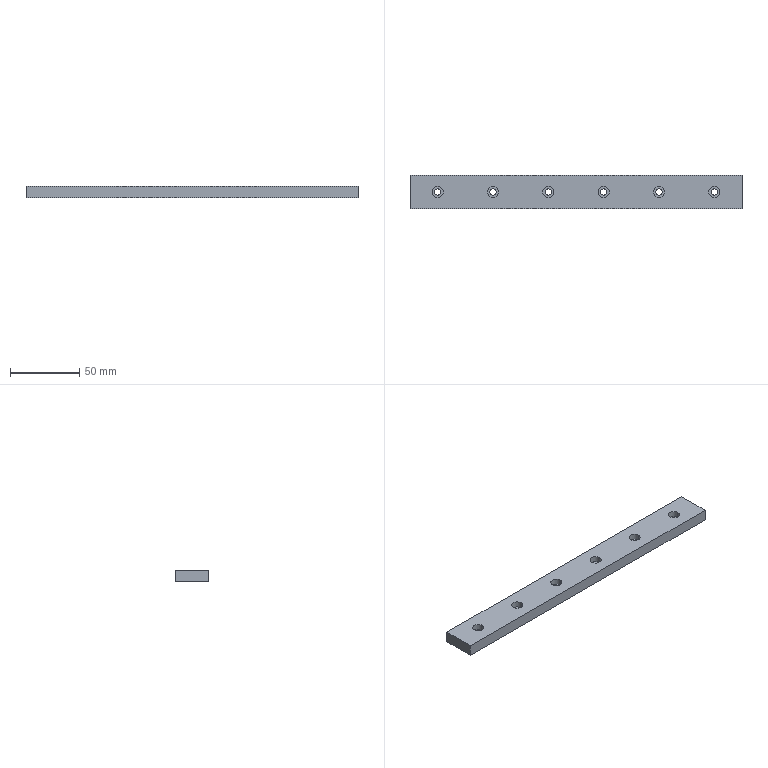Part | SolidWorks | features Extrusion 1, HoleWzd 1, LPattern 1 | 1 solid | 36 faces | box 240 x 24 x 8.5 mm | volume 47242 mm3 | cylinder 24 | plane 12 | commonest cylinder face diameters 4.5 x12 8 x12
STEP:
#1=CARTESIAN_POINT('',(96.,0.,4.1));
#2=VERTEX_POINT('',#1);
#3=CARTESIAN_POINT('',(104.,0.,4.1));
#4=VERTEX_POINT('',#3);
#5=CARTESIAN_POINT('',(100.,0.,4.1));
#6=DIRECTION('',(0.,0.,1.));
#7=DIRECTION('',(1.,0.,0.));
#8=AXIS2_PLACEMENT_3D('',#5,#6,#7);
#9=CIRCLE('',#8,4.);
#10=EDGE_CURVE('',#2,#4,#9,.T.);
#11=ORIENTED_EDGE('',*,*,#10,.F.);
#12=CARTESIAN_POINT('',(96.,0.,8.5));
#13=VERTEX_POINT('',#12);
#14=CARTESIAN_POINT('',(96.,0.,8.5));
#15=DIRECTION('',(0.,0.,1.));
#16=VECTOR('',#15,1000.);
#17=LINE('',#14,#16);
#18=EDGE_CURVE('',#2,#13,#17,.T.);
#19=ORIENTED_EDGE('',*,*,#18,.T.);
#20=CARTESIAN_POINT('',(104.,0.,8.5));
#21=VERTEX_POINT('',#20);
#22=CARTESIAN_POINT('',(100.,0.,8.5));
#23=DIRECTION('',(0.,0.,1.));
#24=DIRECTION('',(1.,0.,0.));
#25=AXIS2_PLACEMENT_3D('',#22,#23,#24);
#26=CIRCLE('',#25,4.);
#27=EDGE_CURVE('',#13,#21,#26,.T.);
#28=ORIENTED_EDGE('',*,*,#27,.T.);
#29=CARTESIAN_POINT('',(104.,0.,8.5));
#30=DIRECTION('',(0.,0.,1.));
#31=VECTOR('',#30,1000.);
#32=LINE('',#29,#31);
#33=EDGE_CURVE('',#4,#21,#32,.T.);
#34=ORIENTED_EDGE('',*,*,#33,.F.);
#35=EDGE_LOOP('',(#11,#19,#28,#34));
#36=FACE_OUTER_BOUND('',#35,.T.);
#37=CARTESIAN_POINT('',(100.,0.,8.5));
#38=DIRECTION('',(0.,0.,1.));
#39=DIRECTION('',(1.,0.,0.));
#40=AXIS2_PLACEMENT_3D('',#37,#38,#39);
#41=CYLINDRICAL_SURFACE('',#40,4.);
#42=ADVANCED_FACE('',(#36),#41,.F.);
#43=CARTESIAN_POINT('',(97.75,0.,0.));
#44=VERTEX_POINT('',#43);
#45=CARTESIAN_POINT('',(102.25,0.,0.));
#46=VERTEX_POINT('',#45);
#47=CARTESIAN_POINT('',(100.,0.,0.));
#48=DIRECTION('',(0.,0.,1.));
#49=DIRECTION('',(1.,0.,0.));
#50=AXIS2_PLACEMENT_3D('',#47,#48,#49);
#51=CIRCLE('',#50,2.25);
#52=EDGE_CURVE('',#44,#46,#51,.T.);
#53=ORIENTED_EDGE('',*,*,#52,.F.);
#54=CARTESIAN_POINT('',(97.75,0.,4.1));
#55=VERTEX_POINT('',#54);
#56=CARTESIAN_POINT('',(97.75,0.,8.5));
#57=DIRECTION('',(0.,0.,1.));
#58=VECTOR('',#57,1000.);
#59=LINE('',#56,#58);
#60=EDGE_CURVE('',#44,#55,#59,.T.);
#61=ORIENTED_EDGE('',*,*,#60,.T.);
#62=CARTESIAN_POINT('',(102.25,0.,4.1));
#63=VERTEX_POINT('',#62);
#64=CARTESIAN_POINT('',(100.,0.,4.1));
#65=DIRECTION('',(0.,0.,1.));
#66=DIRECTION('',(1.,0.,0.));
#67=AXIS2_PLACEMENT_3D('',#64,#65,#66);
#68=CIRCLE('',#67,2.25);
#69=EDGE_CURVE('',#55,#63,#68,.T.);
#70=ORIENTED_EDGE('',*,*,#69,.T.);
#71=CARTESIAN_POINT('',(102.25,0.,8.5));
#72=DIRECTION('',(0.,0.,1.));
#73=VECTOR('',#72,1000.);
#74=LINE('',#71,#73);
#75=EDGE_CURVE('',#46,#63,#74,.T.);
#76=ORIENTED_EDGE('',*,*,#75,.F.);
#77=EDGE_LOOP('',(#53,#61,#70,#76));
#78=FACE_OUTER_BOUND('',#77,.T.);
#79=CARTESIAN_POINT('',(100.,0.,8.5));
#80=DIRECTION('',(0.,0.,1.));
#81=DIRECTION('',(1.,0.,0.));
#82=AXIS2_PLACEMENT_3D('',#79,#80,#81);
#83=CYLINDRICAL_SURFACE('',#82,2.25);
#84=ADVANCED_FACE('',(#78),#83,.F.);
#85=CARTESIAN_POINT('',(56.,0.,4.1));
#86=VERTEX_POINT('',#85);
#87=CARTESIAN_POINT('',(64.,0.,4.1));
#88=VERTEX_POINT('',#87);
#89=CARTESIAN_POINT('',(60.,0.,4.1));
#90=DIRECTION('',(0.,0.,1.));
#91=DIRECTION('',(1.,0.,0.));
#92=AXIS2_PLACEMENT_3D('',#89,#90,#91);
#93=CIRCLE('',#92,4.);
#94=EDGE_CURVE('',#86,#88,#93,.T.);
#95=ORIENTED_EDGE('',*,*,#94,.F.);
#96=CARTESIAN_POINT('',(56.,0.,8.5));
#97=VERTEX_POINT('',#96);
#98=CARTESIAN_POINT('',(56.,0.,8.5));
#99=DIRECTION('',(0.,0.,1.));
#100=VECTOR('',#99,1000.);
#101=LINE('',#98,#100);
#102=EDGE_CURVE('',#86,#97,#101,.T.);
#103=ORIENTED_EDGE('',*,*,#102,.T.);
#104=CARTESIAN_POINT('',(64.,0.,8.5));
#105=VERTEX_POINT('',#104);
#106=CARTESIAN_POINT('',(60.,0.,8.5));
#107=DIRECTION('',(0.,0.,1.));
#108=DIRECTION('',(1.,0.,0.));
#109=AXIS2_PLACEMENT_3D('',#106,#107,#108);
#110=CIRCLE('',#109,4.);
#111=EDGE_CURVE('',#97,#105,#110,.T.);
#112=ORIENTED_EDGE('',*,*,#111,.T.);
#113=CARTESIAN_POINT('',(64.,0.,8.5));
#114=DIRECTION('',(0.,0.,1.));
#115=VECTOR('',#114,1000.);
#116=LINE('',#113,#115);
#117=EDGE_CURVE('',#88,#105,#116,.T.);
#118=ORIENTED_EDGE('',*,*,#117,.F.);
#119=EDGE_LOOP('',(#95,#103,#112,#118));
#120=FACE_OUTER_BOUND('',#119,.T.);
#121=CARTESIAN_POINT('',(60.,0.,8.5));
#122=DIRECTION('',(0.,0.,1.));
#123=DIRECTION('',(1.,0.,0.));
#124=AXIS2_PLACEMENT_3D('',#121,#122,#123);
#125=CYLINDRICAL_SURFACE('',#124,4.);
#126=ADVANCED_FACE('',(#120),#125,.F.);
#127=CARTESIAN_POINT('',(57.75,0.,0.));
#128=VERTEX_POINT('',#127);
#129=CARTESIAN_POINT('',(62.25,0.,0.));
#130=VERTEX_POINT('',#129);
#131=CARTESIAN_POINT('',(60.,0.,0.));
#132=DIRECTION('',(0.,0.,1.));
#133=DIRECTION('',(1.,0.,0.));
#134=AXIS2_PLACEMENT_3D('',#131,#132,#133);
#135=CIRCLE('',#134,2.25);
#136=EDGE_CURVE('',#128,#130,#135,.T.);
#137=ORIENTED_EDGE('',*,*,#136,.F.);
#138=CARTESIAN_POINT('',(57.75,0.,4.1));
#139=VERTEX_POINT('',#138);
#140=CARTESIAN_POINT('',(57.75,0.,8.5));
#141=DIRECTION('',(0.,0.,1.));
#142=VECTOR('',#141,1000.);
#143=LINE('',#140,#142);
#144=EDGE_CURVE('',#128,#139,#143,.T.);
#145=ORIENTED_EDGE('',*,*,#144,.T.);
#146=CARTESIAN_POINT('',(62.25,0.,4.1));
#147=VERTEX_POINT('',#146);
#148=CARTESIAN_POINT('',(60.,0.,4.1));
#149=DIRECTION('',(0.,0.,1.));
#150=DIRECTION('',(1.,0.,0.));
#151=AXIS2_PLACEMENT_3D('',#148,#149,#150);
#152=CIRCLE('',#151,2.25);
#153=EDGE_CURVE('',#139,#147,#152,.T.);
#154=ORIENTED_EDGE('',*,*,#153,.T.);
#155=CARTESIAN_POINT('',(62.25,0.,8.5));
#156=DIRECTION('',(0.,0.,1.));
#157=VECTOR('',#156,1000.);
#158=LINE('',#155,#157);
#159=EDGE_CURVE('',#130,#147,#158,.T.);
#160=ORIENTED_EDGE('',*,*,#159,.F.);
#161=EDGE_LOOP('',(#137,#145,#154,#160));
#162=FACE_OUTER_BOUND('',#161,.T.);
#163=CARTESIAN_POINT('',(60.,0.,8.5));
#164=DIRECTION('',(0.,0.,1.));
#165=DIRECTION('',(1.,0.,0.));
#166=AXIS2_PLACEMENT_3D('',#163,#164,#165);
#167=CYLINDRICAL_SURFACE('',#166,2.25);
#168=ADVANCED_FACE('',(#162),#167,.F.);
#169=CARTESIAN_POINT('',(16.,0.,4.1));
#170=VERTEX_POINT('',#169);
#171=CARTESIAN_POINT('',(24.,0.,4.1));
#172=VERTEX_POINT('',#171);
#173=CARTESIAN_POINT('',(20.,0.,4.1));
#174=DIRECTION('',(0.,0.,1.));
#175=DIRECTION('',(1.,0.,0.));
#176=AXIS2_PLACEMENT_3D('',#173,#174,#175);
#177=CIRCLE('',#176,4.);
#178=EDGE_CURVE('',#170,#172,#177,.T.);
#179=ORIENTED_EDGE('',*,*,#178,.F.);
#180=CARTESIAN_POINT('',(16.,0.,8.5));
#181=VERTEX_POINT('',#180);
#182=CARTESIAN_POINT('',(16.,0.,8.5));
#183=DIRECTION('',(0.,0.,1.));
#184=VECTOR('',#183,1000.);
#185=LINE('',#182,#184);
#186=EDGE_CURVE('',#170,#181,#185,.T.);
#187=ORIENTED_EDGE('',*,*,#186,.T.);
#188=CARTESIAN_POINT('',(24.,0.,8.5));
#189=VERTEX_POINT('',#188);
#190=CARTESIAN_POINT('',(20.,0.,8.5));
#191=DIRECTION('',(0.,0.,1.));
#192=DIRECTION('',(1.,0.,0.));
#193=AXIS2_PLACEMENT_3D('',#190,#191,#192);
#194=CIRCLE('',#193,4.);
#195=EDGE_CURVE('',#181,#189,#194,.T.);
#196=ORIENTED_EDGE('',*,*,#195,.T.);
#197=CARTESIAN_POINT('',(24.,0.,8.5));
#198=DIRECTION('',(0.,0.,1.));
#199=VECTOR('',#198,1000.);
#200=LINE('',#197,#199);
#201=EDGE_CURVE('',#172,#189,#200,.T.);
#202=ORIENTED_EDGE('',*,*,#201,.F.);
#203=EDGE_LOOP('',(#179,#187,#196,#202));
#204=FACE_OUTER_BOUND('',#203,.T.);
#205=CARTESIAN_POINT('',(20.,0.,8.5));
#206=DIRECTION('',(0.,0.,1.));
#207=DIRECTION('',(1.,0.,0.));
#208=AXIS2_PLACEMENT_3D('',#205,#206,#207);
#209=CYLINDRICAL_SURFACE('',#208,4.);
#210=ADVANCED_FACE('',(#204),#209,.F.);
#211=CARTESIAN_POINT('',(17.75,0.,0.));
#212=VERTEX_POINT('',#211);
#213=CARTESIAN_POINT('',(22.25,0.,0.));
#214=VERTEX_POINT('',#213);
#215=CARTESIAN_POINT('',(20.,0.,0.));
#216=DIRECTION('',(0.,0.,1.));
#217=DIRECTION('',(1.,0.,0.));
#218=AXIS2_PLACEMENT_3D('',#215,#216,#217);
#219=CIRCLE('',#218,2.25);
#220=EDGE_CURVE('',#212,#214,#219,.T.);
#221=ORIENTED_EDGE('',*,*,#220,.F.);
#222=CARTESIAN_POINT('',(17.75,0.,4.1));
#223=VERTEX_POINT('',#222);
#224=CARTESIAN_POINT('',(17.75,0.,8.5));
#225=DIRECTION('',(0.,0.,1.));
#226=VECTOR('',#225,1000.);
#227=LINE('',#224,#226);
#228=EDGE_CURVE('',#212,#223,#227,.T.);
#229=ORIENTED_EDGE('',*,*,#228,.T.);
#230=CARTESIAN_POINT('',(22.25,0.,4.1));
#231=VERTEX_POINT('',#230);
#232=CARTESIAN_POINT('',(20.,0.,4.1));
#233=DIRECTION('',(0.,0.,1.));
#234=DIRECTION('',(1.,0.,0.));
#235=AXIS2_PLACEMENT_3D('',#232,#233,#234);
#236=CIRCLE('',#235,2.25);
#237=EDGE_CURVE('',#223,#231,#236,.T.);
#238=ORIENTED_EDGE('',*,*,#237,.T.);
#239=CARTESIAN_POINT('',(22.25,0.,8.5));
#240=DIRECTION('',(0.,0.,1.));
#241=VECTOR('',#240,1000.);
#242=LINE('',#239,#241);
#243=EDGE_CURVE('',#214,#231,#242,.T.);
#244=ORIENTED_EDGE('',*,*,#243,.F.);
#245=EDGE_LOOP('',(#221,#229,#238,#244));
#246=FACE_OUTER_BOUND('',#245,.T.);
#247=CARTESIAN_POINT('',(20.,0.,8.5));
#248=DIRECTION('',(0.,0.,1.));
#249=DIRECTION('',(1.,0.,0.));
#250=AXIS2_PLACEMENT_3D('',#247,#248,#249);
#251=CYLINDRICAL_SURFACE('',#250,2.25);
#252=ADVANCED_FACE('',(#246),#251,.F.);
#253=CARTESIAN_POINT('',(-24.,0.,4.1));
#254=VERTEX_POINT('',#253);
#255=CARTESIAN_POINT('',(-16.,0.,4.1));
#256=VERTEX_POINT('',#255);
#257=CARTESIAN_POINT('',(-20.,0.,4.1));
#258=DIRECTION('',(0.,0.,1.));
#259=DIRECTION('',(1.,0.,0.));
#260=AXIS2_PLACEMENT_3D('',#257,#258,#259);
#261=CIRCLE('',#260,4.);
#262=EDGE_CURVE('',#254,#256,#261,.T.);
#263=ORIENTED_EDGE('',*,*,#262,.F.);
#264=CARTESIAN_POINT('',(-24.,0.,8.5));
#265=VERTEX_POINT('',#264);
#266=CARTESIAN_POINT('',(-24.,0.,8.5));
#267=DIRECTION('',(0.,0.,1.));
#268=VECTOR('',#267,1000.);
#269=LINE('',#266,#268);
#270=EDGE_CURVE('',#254,#265,#269,.T.);
#271=ORIENTED_EDGE('',*,*,#270,.T.);
#272=CARTESIAN_POINT('',(-16.,0.,8.5));
#273=VERTEX_POINT('',#272);
#274=CARTESIAN_POINT('',(-20.,0.,8.5));
#275=DIRECTION('',(0.,0.,1.));
#276=DIRECTION('',(1.,0.,0.));
#277=AXIS2_PLACEMENT_3D('',#274,#275,#276);
#278=CIRCLE('',#277,4.);
#279=EDGE_CURVE('',#265,#273,#278,.T.);
#280=ORIENTED_EDGE('',*,*,#279,.T.);
#281=CARTESIAN_POINT('',(-16.,0.,8.5));
#282=DIRECTION('',(0.,0.,1.));
#283=VECTOR('',#282,1000.);
#284=LINE('',#281,#283);
#285=EDGE_CURVE('',#256,#273,#284,.T.);
#286=ORIENTED_EDGE('',*,*,#285,.F.);
#287=EDGE_LOOP('',(#263,#271,#280,#286));
#288=FACE_OUTER_BOUND('',#287,.T.);
#289=CARTESIAN_POINT('',(-20.,0.,8.5));
#290=DIRECTION('',(0.,0.,1.));
#291=DIRECTION('',(1.,0.,0.));
#292=AXIS2_PLACEMENT_3D('',#289,#290,#291);
#293=CYLINDRICAL_SURFACE('',#292,4.);
#294=ADVANCED_FACE('',(#288),#293,.F.);
#295=CARTESIAN_POINT('',(-22.25,0.,0.));
#296=VERTEX_POINT('',#295);
#297=CARTESIAN_POINT('',(-17.75,0.,0.));
#298=VERTEX_POINT('',#297);
#299=CARTESIAN_POINT('',(-20.,0.,0.));
#300=DIRECTION('',(0.,0.,1.));
#301=DIRECTION('',(1.,0.,0.));
#302=AXIS2_PLACEMENT_3D('',#299,#300,#301);
#303=CIRCLE('',#302,2.25);
#304=EDGE_CURVE('',#296,#298,#303,.T.);
#305=ORIENTED_EDGE('',*,*,#304,.F.);
#306=CARTESIAN_POINT('',(-22.25,0.,4.1));
#307=VERTEX_POINT('',#306);
#308=CARTESIAN_POINT('',(-22.25,0.,8.5));
#309=DIRECTION('',(0.,0.,1.));
#310=VECTOR('',#309,1000.);
#311=LINE('',#308,#310);
#312=EDGE_CURVE('',#296,#307,#311,.T.);
#313=ORIENTED_EDGE('',*,*,#312,.T.);
#314=CARTESIAN_POINT('',(-17.75,0.,4.1));
#315=VERTEX_POINT('',#314);
#316=CARTESIAN_POINT('',(-20.,0.,4.1));
#317=DIRECTION('',(0.,0.,1.));
#318=DIRECTION('',(1.,0.,0.));
#319=AXIS2_PLACEMENT_3D('',#316,#317,#318);
#320=CIRCLE('',#319,2.25);
#321=EDGE_CURVE('',#307,#315,#320,.T.);
#322=ORIENTED_EDGE('',*,*,#321,.T.);
#323=CARTESIAN_POINT('',(-17.75,0.,8.5));
#324=DIRECTION('',(0.,0.,1.));
#325=VECTOR('',#324,1000.);
#326=LINE('',#323,#325);
#327=EDGE_CURVE('',#298,#315,#326,.T.);
#328=ORIENTED_EDGE('',*,*,#327,.F.);
#329=EDGE_LOOP('',(#305,#313,#322,#328));
#330=FACE_OUTER_BOUND('',#329,.T.);
#331=CARTESIAN_POINT('',(-20.,0.,8.5));
#332=DIRECTION('',(0.,0.,1.));
#333=DIRECTION('',(1.,0.,0.));
#334=AXIS2_PLACEMENT_3D('',#331,#332,#333);
#335=CYLINDRICAL_SURFACE('',#334,2.25);
#336=ADVANCED_FACE('',(#330),#335,.F.);
#337=CARTESIAN_POINT('',(-64.,0.,4.1));
#338=VERTEX_POINT('',#337);
#339=CARTESIAN_POINT('',(-56.,0.,4.1));
#340=VERTEX_POINT('',#339);
#341=CARTESIAN_POINT('',(-60.,0.,4.1));
#342=DIRECTION('',(0.,0.,1.));
#343=DIRECTION('',(1.,0.,0.));
#344=AXIS2_PLACEMENT_3D('',#341,#342,#343);
#345=CIRCLE('',#344,4.);
#346=EDGE_CURVE('',#338,#340,#345,.T.);
#347=ORIENTED_EDGE('',*,*,#346,.F.);
#348=CARTESIAN_POINT('',(-64.,0.,8.5));
#349=VERTEX_POINT('',#348);
#350=CARTESIAN_POINT('',(-64.,0.,8.5));
#351=DIRECTION('',(0.,0.,1.));
#352=VECTOR('',#351,1000.);
#353=LINE('',#350,#352);
#354=EDGE_CURVE('',#338,#349,#353,.T.);
#355=ORIENTED_EDGE('',*,*,#354,.T.);
#356=CARTESIAN_POINT('',(-56.,0.,8.5));
#357=VERTEX_POINT('',#356);
#358=CARTESIAN_POINT('',(-60.,0.,8.5));
#359=DIRECTION('',(0.,0.,1.));
#360=DIRECTION('',(1.,0.,0.));
#361=AXIS2_PLACEMENT_3D('',#358,#359,#360);
#362=CIRCLE('',#361,4.);
#363=EDGE_CURVE('',#349,#357,#362,.T.);
#364=ORIENTED_EDGE('',*,*,#363,.T.);
#365=CARTESIAN_POINT('',(-56.,0.,8.5));
#366=DIRECTION('',(0.,0.,1.));
#367=VECTOR('',#366,1000.);
#368=LINE('',#365,#367);
#369=EDGE_CURVE('',#340,#357,#368,.T.);
#370=ORIENTED_EDGE('',*,*,#369,.F.);
#371=EDGE_LOOP('',(#347,#355,#364,#370));
#372=FACE_OUTER_BOUND('',#371,.T.);
#373=CARTESIAN_POINT('',(-60.,0.,8.5));
#374=DIRECTION('',(0.,0.,1.));
#375=DIRECTION('',(1.,0.,0.));
#376=AXIS2_PLACEMENT_3D('',#373,#374,#375);
#377=CYLINDRICAL_SURFACE('',#376,4.);
#378=ADVANCED_FACE('',(#372),#377,.F.);
#379=CARTESIAN_POINT('',(-62.25,0.,0.));
#380=VERTEX_POINT('',#379);
#381=CARTESIAN_POINT('',(-57.75,0.,0.));
#382=VERTEX_POINT('',#381);
#383=CARTESIAN_POINT('',(-60.,0.,0.));
#384=DIRECTION('',(0.,0.,1.));
#385=DIRECTION('',(1.,0.,0.));
#386=AXIS2_PLACEMENT_3D('',#383,#384,#385);
#387=CIRCLE('',#386,2.25);
#388=EDGE_CURVE('',#380,#382,#387,.T.);
#389=ORIENTED_EDGE('',*,*,#388,.F.);
#390=CARTESIAN_POINT('',(-62.25,0.,4.1));
#391=VERTEX_POINT('',#390);
#392=CARTESIAN_POINT('',(-62.25,0.,8.5));
#393=DIRECTION('',(0.,0.,1.));
#394=VECTOR('',#393,1000.);
#395=LINE('',#392,#394);
#396=EDGE_CURVE('',#380,#391,#395,.T.);
#397=ORIENTED_EDGE('',*,*,#396,.T.);
#398=CARTESIAN_POINT('',(-57.75,0.,4.1));
#399=VERTEX_POINT('',#398);
#400=CARTESIAN_POINT('',(-60.,0.,4.1));
#401=DIRECTION('',(0.,0.,1.));
#402=DIRECTION('',(1.,0.,0.));
#403=AXIS2_PLACEMENT_3D('',#400,#401,#402);
#404=CIRCLE('',#403,2.25);
#405=EDGE_CURVE('',#391,#399,#404,.T.);
#406=ORIENTED_EDGE('',*,*,#405,.T.);
#407=CARTESIAN_POINT('',(-57.75,0.,8.5));
#408=DIRECTION('',(0.,0.,1.));
#409=VECTOR('',#408,1000.);
#410=LINE('',#407,#409);
#411=EDGE_CURVE('',#382,#399,#410,.T.);
#412=ORIENTED_EDGE('',*,*,#411,.F.);
#413=EDGE_LOOP('',(#389,#397,#406,#412));
#414=FACE_OUTER_BOUND('',#413,.T.);
#415=CARTESIAN_POINT('',(-60.,0.,8.5));
#416=DIRECTION('',(0.,0.,1.));
#417=DIRECTION('',(1.,0.,0.));
#418=AXIS2_PLACEMENT_3D('',#415,#416,#417);
#419=CYLINDRICAL_SURFACE('',#418,2.25);
#420=ADVANCED_FACE('',(#414),#419,.F.);
#421=CARTESIAN_POINT('',(-104.,0.,4.1));
#422=VERTEX_POINT('',#421);
#423=CARTESIAN_POINT('',(-96.,0.,4.1));
#424=VERTEX_POINT('',#423);
#425=CARTESIAN_POINT('',(-100.,0.,4.1));
#426=DIRECTION('',(0.,0.,1.));
#427=DIRECTION('',(1.,0.,0.));
#428=AXIS2_PLACEMENT_3D('',#425,#426,#427);
#429=CIRCLE('',#428,4.);
#430=EDGE_CURVE('',#422,#424,#429,.T.);
#431=ORIENTED_EDGE('',*,*,#430,.F.);
#432=CARTESIAN_POINT('',(-104.,0.,8.5));
#433=VERTEX_POINT('',#432);
#434=CARTESIAN_POINT('',(-104.,0.,8.5));
#435=DIRECTION('',(0.,0.,1.));
#436=VECTOR('',#435,1000.);
#437=LINE('',#434,#436);
#438=EDGE_CURVE('',#422,#433,#437,.T.);
#439=ORIENTED_EDGE('',*,*,#438,.T.);
#440=CARTESIAN_POINT('',(-96.,0.,8.5));
#441=VERTEX_POINT('',#440);
#442=CARTESIAN_POINT('',(-100.,0.,8.5));
#443=DIRECTION('',(0.,0.,1.));
#444=DIRECTION('',(1.,0.,0.));
#445=AXIS2_PLACEMENT_3D('',#442,#443,#444);
#446=CIRCLE('',#445,4.);
#447=EDGE_CURVE('',#433,#441,#446,.T.);
#448=ORIENTED_EDGE('',*,*,#447,.T.);
#449=CARTESIAN_POINT('',(-96.,0.,8.5));
#450=DIRECTION('',(0.,0.,1.));
#451=VECTOR('',#450,1000.);
#452=LINE('',#449,#451);
#453=EDGE_CURVE('',#424,#441,#452,.T.);
#454=ORIENTED_EDGE('',*,*,#453,.F.);
#455=EDGE_LOOP('',(#431,#439,#448,#454));
#456=FACE_OUTER_BOUND('',#455,.T.);
#457=CARTESIAN_POINT('',(-100.,0.,8.5));
#458=DIRECTION('',(0.,0.,1.));
#459=DIRECTION('',(1.,0.,0.));
#460=AXIS2_PLACEMENT_3D('',#457,#458,#459);
#461=CYLINDRICAL_SURFACE('',#460,4.);
#462=ADVANCED_FACE('',(#456),#461,.F.);
#463=CARTESIAN_POINT('',(-102.25,0.,0.));
#464=VERTEX_POINT('',#463);
#465=CARTESIAN_POINT('',(-97.75,0.,0.));
#466=VERTEX_POINT('',#465);
#467=CARTESIAN_POINT('',(-100.,0.,0.));
#468=DIRECTION('',(0.,0.,1.));
#469=DIRECTION('',(1.,0.,0.));
#470=AXIS2_PLACEMENT_3D('',#467,#468,#469);
#471=CIRCLE('',#470,2.25);
#472=EDGE_CURVE('',#464,#466,#471,.T.);
#473=ORIENTED_EDGE('',*,*,#472,.F.);
#474=CARTESIAN_POINT('',(-102.25,0.,4.1));
#475=VERTEX_POINT('',#474);
#476=CARTESIAN_POINT('',(-102.25,0.,8.5));
#477=DIRECTION('',(0.,0.,1.));
#478=VECTOR('',#477,1000.);
#479=LINE('',#476,#478);
#480=EDGE_CURVE('',#464,#475,#479,.T.);
#481=ORIENTED_EDGE('',*,*,#480,.T.);
#482=CARTESIAN_POINT('',(-97.75,0.,4.1));
#483=VERTEX_POINT('',#482);
#484=CARTESIAN_POINT('',(-100.,0.,4.1));
#485=DIRECTION('',(0.,0.,1.));
#486=DIRECTION('',(1.,0.,0.));
#487=AXIS2_PLACEMENT_3D('',#484,#485,#486);
#488=CIRCLE('',#487,2.25);
#489=EDGE_CURVE('',#475,#483,#488,.T.);
#490=ORIENTED_EDGE('',*,*,#489,.T.);
#491=CARTESIAN_POINT('',(-97.75,0.,8.5));
#492=DIRECTION('',(0.,0.,1.));
#493=VECTOR('',#492,1000.);
#494=LINE('',#491,#493);
#495=EDGE_CURVE('',#466,#483,#494,.T.);
#496=ORIENTED_EDGE('',*,*,#495,.F.);
#497=EDGE_LOOP('',(#473,#481,#490,#496));
#498=FACE_OUTER_BOUND('',#497,.T.);
#499=CARTESIAN_POINT('',(-100.,0.,8.5));
#500=DIRECTION('',(0.,0.,1.));
#501=DIRECTION('',(1.,0.,0.));
#502=AXIS2_PLACEMENT_3D('',#499,#500,#501);
#503=CYLINDRICAL_SURFACE('',#502,2.25);
#504=ADVANCED_FACE('',(#498),#503,.F.);
#505=CARTESIAN_POINT('',(120.,-12.,0.));
#506=VERTEX_POINT('',#505);
#507=CARTESIAN_POINT('',(120.,12.,0.));
#508=VERTEX_POINT('',#507);
#509=CARTESIAN_POINT('',(120.,12.,0.));
#510=DIRECTION('',(0.,1.,0.));
#511=VECTOR('',#510,1000.);
#512=LINE('',#509,#511);
#513=EDGE_CURVE('',#506,#508,#512,.T.);
#514=ORIENTED_EDGE('',*,*,#513,.T.);
#515=CARTESIAN_POINT('',(120.,12.,8.5));
#516=VERTEX_POINT('',#515);
#517=CARTESIAN_POINT('',(120.,12.,8.5));
#518=DIRECTION('',(0.,0.,-1.));
#519=VECTOR('',#518,1000.);
#520=LINE('',#517,#519);
#521=EDGE_CURVE('',#516,#508,#520,.T.);
#522=ORIENTED_EDGE('',*,*,#521,.F.);
#523=CARTESIAN_POINT('',(120.,-12.,8.5));
#524=VERTEX_POINT('',#523);
#525=CARTESIAN_POINT('',(120.,12.,8.5));
#526=DIRECTION('',(0.,1.,0.));
#527=VECTOR('',#526,1000.);
#528=LINE('',#525,#527);
#529=EDGE_CURVE('',#524,#516,#528,.T.);
#530=ORIENTED_EDGE('',*,*,#529,.F.);
#531=CARTESIAN_POINT('',(120.,-12.,8.5));
#532=DIRECTION('',(0.,0.,-1.));
#533=VECTOR('',#532,1000.);
#534=LINE('',#531,#533);
#535=EDGE_CURVE('',#524,#506,#534,.T.);
#536=ORIENTED_EDGE('',*,*,#535,.T.);
#537=EDGE_LOOP('',(#514,#522,#530,#536));
#538=FACE_OUTER_BOUND('',#537,.T.);
#539=CARTESIAN_POINT('',(120.,12.,8.5));
#540=DIRECTION('',(-1.,0.,0.));
#541=DIRECTION('',(0.,0.,1.));
#542=AXIS2_PLACEMENT_3D('',#539,#540,#541);
#543=PLANE('',#542);
#544=ADVANCED_FACE('',(#538),#543,.F.);
#545=CARTESIAN_POINT('',(-120.,12.,0.));
#546=VERTEX_POINT('',#545);
#547=CARTESIAN_POINT('',(-120.,12.,0.));
#548=DIRECTION('',(-1.,0.,0.));
#549=VECTOR('',#548,1000.);
#550=LINE('',#547,#549);
#551=EDGE_CURVE('',#508,#546,#550,.T.);
#552=ORIENTED_EDGE('',*,*,#551,.T.);
#553=CARTESIAN_POINT('',(-120.,12.,8.5));
#554=VERTEX_POINT('',#553);
#555=CARTESIAN_POINT('',(-120.,12.,8.5));
#556=DIRECTION('',(0.,0.,-1.));
#557=VECTOR('',#556,1000.);
#558=LINE('',#555,#557);
#559=EDGE_CURVE('',#554,#546,#558,.T.);
#560=ORIENTED_EDGE('',*,*,#559,.F.);
#561=CARTESIAN_POINT('',(-120.,12.,8.5));
#562=DIRECTION('',(-1.,0.,0.));
#563=VECTOR('',#562,1000.);
#564=LINE('',#561,#563);
#565=EDGE_CURVE('',#516,#554,#564,.T.);
#566=ORIENTED_EDGE('',*,*,#565,.F.);
#567=ORIENTED_EDGE('',*,*,#521,.T.);
#568=EDGE_LOOP('',(#552,#560,#566,#567));
#569=FACE_OUTER_BOUND('',#568,.T.);
#570=CARTESIAN_POINT('',(-120.,12.,8.5));
#571=DIRECTION('',(0.,-1.,0.));
#572=DIRECTION('',(0.,0.,-1.));
#573=AXIS2_PLACEMENT_3D('',#570,#571,#572);
#574=PLANE('',#573);
#575=ADVANCED_FACE('',(#569),#574,.F.);
#576=CARTESIAN_POINT('',(-120.,-12.,0.));
#577=VERTEX_POINT('',#576);
#578=CARTESIAN_POINT('',(-120.,12.,0.));
#579=DIRECTION('',(0.,-1.,0.));
#580=VECTOR('',#579,1000.);
#581=LINE('',#578,#580);
#582=EDGE_CURVE('',#546,#577,#581,.T.);
#583=ORIENTED_EDGE('',*,*,#582,.T.);
#584=CARTESIAN_POINT('',(-120.,-12.,8.5));
#585=VERTEX_POINT('',#584);
#586=CARTESIAN_POINT('',(-120.,-12.,8.5));
#587=DIRECTION('',(0.,0.,-1.));
#588=VECTOR('',#587,1000.);
#589=LINE('',#586,#588);
#590=EDGE_CURVE('',#585,#577,#589,.T.);
#591=ORIENTED_EDGE('',*,*,#590,.F.);
#592=CARTESIAN_POINT('',(-120.,12.,8.5));
#593=DIRECTION('',(0.,-1.,0.));
#594=VECTOR('',#593,1000.);
#595=LINE('',#592,#594);
#596=EDGE_CURVE('',#554,#585,#595,.T.);
#597=ORIENTED_EDGE('',*,*,#596,.F.);
#598=ORIENTED_EDGE('',*,*,#559,.T.);
#599=EDGE_LOOP('',(#583,#591,#597,#598));
#600=FACE_OUTER_BOUND('',#599,.T.);
#601=CARTESIAN_POINT('',(-120.,12.,8.5));
#602=DIRECTION('',(1.,0.,0.));
#603=DIRECTION('',(0.,0.,-1.));
#604=AXIS2_PLACEMENT_3D('',#601,#602,#603);
#605=PLANE('',#604);
#606=ADVANCED_FACE('',(#600),#605,.F.);
#607=CARTESIAN_POINT('',(-120.,-12.,0.));
#608=DIRECTION('',(1.,0.,0.));
#609=VECTOR('',#608,1000.);
#610=LINE('',#607,#609);
#611=EDGE_CURVE('',#577,#506,#610,.T.);
#612=ORIENTED_EDGE('',*,*,#611,.T.);
#613=ORIENTED_EDGE('',*,*,#535,.F.);
#614=CARTESIAN_POINT('',(-120.,-12.,8.5));
#615=DIRECTION('',(1.,0.,0.));
#616=VECTOR('',#615,1000.);
#617=LINE('',#614,#616);
#618=EDGE_CURVE('',#585,#524,#617,.T.);
#619=ORIENTED_EDGE('',*,*,#618,.F.);
#620=ORIENTED_EDGE('',*,*,#590,.T.);
#621=EDGE_LOOP('',(#612,#613,#619,#620));
#622=FACE_OUTER_BOUND('',#621,.T.);
#623=CARTESIAN_POINT('',(-120.,-12.,8.5));
#624=DIRECTION('',(0.,1.,0.));
#625=DIRECTION('',(0.,0.,1.));
#626=AXIS2_PLACEMENT_3D('',#623,#624,#625);
#627=PLANE('',#626);
#628=ADVANCED_FACE('',(#622),#627,.F.);
#629=CARTESIAN_POINT('',(100.,0.,8.5));
#630=DIRECTION('',(0.,0.,1.));
#631=DIRECTION('',(1.,0.,0.));
#632=AXIS2_PLACEMENT_3D('',#629,#630,#631);
#633=CIRCLE('',#632,4.);
#634=EDGE_CURVE('',#21,#13,#633,.T.);
#635=ORIENTED_EDGE('',*,*,#634,.F.);
#636=ORIENTED_EDGE('',*,*,#27,.F.);
#637=EDGE_LOOP('',(#635,#636));
#638=FACE_BOUND('',#637,.T.);
#639=CARTESIAN_POINT('',(60.,0.,8.5));
#640=DIRECTION('',(0.,0.,1.));
#641=DIRECTION('',(1.,0.,0.));
#642=AXIS2_PLACEMENT_3D('',#639,#640,#641);
#643=CIRCLE('',#642,4.);
#644=EDGE_CURVE('',#105,#97,#643,.T.);
#645=ORIENTED_EDGE('',*,*,#644,.F.);
#646=ORIENTED_EDGE('',*,*,#111,.F.);
#647=EDGE_LOOP('',(#645,#646));
#648=FACE_BOUND('',#647,.T.);
#649=CARTESIAN_POINT('',(20.,0.,8.5));
#650=DIRECTION('',(0.,0.,1.));
#651=DIRECTION('',(1.,0.,0.));
#652=AXIS2_PLACEMENT_3D('',#649,#650,#651);
#653=CIRCLE('',#652,4.);
#654=EDGE_CURVE('',#189,#181,#653,.T.);
#655=ORIENTED_EDGE('',*,*,#654,.F.);
#656=ORIENTED_EDGE('',*,*,#195,.F.);
#657=EDGE_LOOP('',(#655,#656));
#658=FACE_BOUND('',#657,.T.);
#659=CARTESIAN_POINT('',(-20.,0.,8.5));
#660=DIRECTION('',(0.,0.,1.));
#661=DIRECTION('',(1.,0.,0.));
#662=AXIS2_PLACEMENT_3D('',#659,#660,#661);
#663=CIRCLE('',#662,4.);
#664=EDGE_CURVE('',#273,#265,#663,.T.);
#665=ORIENTED_EDGE('',*,*,#664,.F.);
#666=ORIENTED_EDGE('',*,*,#279,.F.);
#667=EDGE_LOOP('',(#665,#666));
#668=FACE_BOUND('',#667,.T.);
#669=CARTESIAN_POINT('',(-60.,0.,8.5));
#670=DIRECTION('',(0.,0.,1.));
#671=DIRECTION('',(1.,0.,0.));
#672=AXIS2_PLACEMENT_3D('',#669,#670,#671);
#673=CIRCLE('',#672,4.);
#674=EDGE_CURVE('',#357,#349,#673,.T.);
#675=ORIENTED_EDGE('',*,*,#674,.F.);
#676=ORIENTED_EDGE('',*,*,#363,.F.);
#677=EDGE_LOOP('',(#675,#676));
#678=FACE_BOUND('',#677,.T.);
#679=CARTESIAN_POINT('',(-100.,0.,8.5));
#680=DIRECTION('',(0.,0.,1.));
#681=DIRECTION('',(1.,0.,0.));
#682=AXIS2_PLACEMENT_3D('',#679,#680,#681);
#683=CIRCLE('',#682,4.);
#684=EDGE_CURVE('',#441,#433,#683,.T.);
#685=ORIENTED_EDGE('',*,*,#684,.F.);
#686=ORIENTED_EDGE('',*,*,#447,.F.);
#687=EDGE_LOOP('',(#685,#686));
#688=FACE_BOUND('',#687,.T.);
#689=ORIENTED_EDGE('',*,*,#529,.T.);
#690=ORIENTED_EDGE('',*,*,#565,.T.);
#691=ORIENTED_EDGE('',*,*,#596,.T.);
#692=ORIENTED_EDGE('',*,*,#618,.T.);
#693=EDGE_LOOP('',(#689,#690,#691,#692));
#694=FACE_OUTER_BOUND('',#693,.T.);
#695=CARTESIAN_POINT('',(0.,0.,8.5));
#696=DIRECTION('',(0.,0.,1.));
#697=DIRECTION('',(1.,0.,0.));
#698=AXIS2_PLACEMENT_3D('',#695,#696,#697);
#699=PLANE('',#698);
#700=ADVANCED_FACE('',(#638,#648,#658,#668,#678,#688,#694),#699,.T.);
#701=CARTESIAN_POINT('',(100.,0.,0.));
#702=DIRECTION('',(0.,0.,1.));
#703=DIRECTION('',(1.,0.,0.));
#704=AXIS2_PLACEMENT_3D('',#701,#702,#703);
#705=CIRCLE('',#704,2.25);
#706=EDGE_CURVE('',#46,#44,#705,.T.);
#707=ORIENTED_EDGE('',*,*,#706,.T.);
#708=ORIENTED_EDGE('',*,*,#52,.T.);
#709=EDGE_LOOP('',(#707,#708));
#710=FACE_BOUND('',#709,.T.);
#711=CARTESIAN_POINT('',(60.,0.,0.));
#712=DIRECTION('',(0.,0.,1.));
#713=DIRECTION('',(1.,0.,0.));
#714=AXIS2_PLACEMENT_3D('',#711,#712,#713);
#715=CIRCLE('',#714,2.25);
#716=EDGE_CURVE('',#130,#128,#715,.T.);
#717=ORIENTED_EDGE('',*,*,#716,.T.);
#718=ORIENTED_EDGE('',*,*,#136,.T.);
#719=EDGE_LOOP('',(#717,#718));
#720=FACE_BOUND('',#719,.T.);
#721=CARTESIAN_POINT('',(20.,0.,0.));
#722=DIRECTION('',(0.,0.,1.));
#723=DIRECTION('',(1.,0.,0.));
#724=AXIS2_PLACEMENT_3D('',#721,#722,#723);
#725=CIRCLE('',#724,2.25);
#726=EDGE_CURVE('',#214,#212,#725,.T.);
#727=ORIENTED_EDGE('',*,*,#726,.T.);
#728=ORIENTED_EDGE('',*,*,#220,.T.);
#729=EDGE_LOOP('',(#727,#728));
#730=FACE_BOUND('',#729,.T.);
#731=CARTESIAN_POINT('',(-20.,0.,0.));
#732=DIRECTION('',(0.,0.,1.));
#733=DIRECTION('',(1.,0.,0.));
#734=AXIS2_PLACEMENT_3D('',#731,#732,#733);
#735=CIRCLE('',#734,2.25);
#736=EDGE_CURVE('',#298,#296,#735,.T.);
#737=ORIENTED_EDGE('',*,*,#736,.T.);
#738=ORIENTED_EDGE('',*,*,#304,.T.);
#739=EDGE_LOOP('',(#737,#738));
#740=FACE_BOUND('',#739,.T.);
#741=CARTESIAN_POINT('',(-60.,0.,0.));
#742=DIRECTION('',(0.,0.,1.));
#743=DIRECTION('',(1.,0.,0.));
#744=AXIS2_PLACEMENT_3D('',#741,#742,#743);
#745=CIRCLE('',#744,2.25);
#746=EDGE_CURVE('',#382,#380,#745,.T.);
#747=ORIENTED_EDGE('',*,*,#746,.T.);
#748=ORIENTED_EDGE('',*,*,#388,.T.);
#749=EDGE_LOOP('',(#747,#748));
#750=FACE_BOUND('',#749,.T.);
#751=CARTESIAN_POINT('',(-100.,0.,0.));
#752=DIRECTION('',(0.,0.,1.));
#753=DIRECTION('',(1.,0.,0.));
#754=AXIS2_PLACEMENT_3D('',#751,#752,#753);
#755=CIRCLE('',#754,2.25);
#756=EDGE_CURVE('',#466,#464,#755,.T.);
#757=ORIENTED_EDGE('',*,*,#756,.T.);
#758=ORIENTED_EDGE('',*,*,#472,.T.);
#759=EDGE_LOOP('',(#757,#758));
#760=FACE_BOUND('',#759,.T.);
#761=ORIENTED_EDGE('',*,*,#513,.F.);
#762=ORIENTED_EDGE('',*,*,#611,.F.);
#763=ORIENTED_EDGE('',*,*,#582,.F.);
#764=ORIENTED_EDGE('',*,*,#551,.F.);
#765=EDGE_LOOP('',(#761,#762,#763,#764));
#766=FACE_OUTER_BOUND('',#765,.T.);
#767=CARTESIAN_POINT('',(0.,0.,0.));
#768=DIRECTION('',(0.,0.,1.));
#769=DIRECTION('',(1.,0.,0.));
#770=AXIS2_PLACEMENT_3D('',#767,#768,#769);
#771=PLANE('',#770);
#772=ADVANCED_FACE('',(#710,#720,#730,#740,#750,#760,#766),#771,.F.);
#773=ORIENTED_EDGE('',*,*,#480,.F.);
#774=ORIENTED_EDGE('',*,*,#756,.F.);
#775=ORIENTED_EDGE('',*,*,#495,.T.);
#776=CARTESIAN_POINT('',(-100.,0.,4.1));
#777=DIRECTION('',(0.,0.,1.));
#778=DIRECTION('',(1.,0.,0.));
#779=AXIS2_PLACEMENT_3D('',#776,#777,#778);
#780=CIRCLE('',#779,2.25);
#781=EDGE_CURVE('',#483,#475,#780,.T.);
#782=ORIENTED_EDGE('',*,*,#781,.T.);
#783=EDGE_LOOP('',(#773,#774,#775,#782));
#784=FACE_OUTER_BOUND('',#783,.T.);
#785=CARTESIAN_POINT('',(-100.,0.,8.5));
#786=DIRECTION('',(0.,0.,1.));
#787=DIRECTION('',(1.,0.,0.));
#788=AXIS2_PLACEMENT_3D('',#785,#786,#787);
#789=CYLINDRICAL_SURFACE('',#788,2.25);
#790=ADVANCED_FACE('',(#784),#789,.F.);
#791=ORIENTED_EDGE('',*,*,#781,.F.);
#792=ORIENTED_EDGE('',*,*,#489,.F.);
#793=EDGE_LOOP('',(#791,#792));
#794=FACE_BOUND('',#793,.T.);
#795=CARTESIAN_POINT('',(-100.,0.,4.1));
#796=DIRECTION('',(0.,0.,1.));
#797=DIRECTION('',(1.,0.,0.));
#798=AXIS2_PLACEMENT_3D('',#795,#796,#797);
#799=CIRCLE('',#798,4.);
#800=EDGE_CURVE('',#424,#422,#799,.T.);
#801=ORIENTED_EDGE('',*,*,#800,.T.);
#802=ORIENTED_EDGE('',*,*,#430,.T.);
#803=EDGE_LOOP('',(#801,#802));
#804=FACE_OUTER_BOUND('',#803,.T.);
#805=CARTESIAN_POINT('',(-97.75,0.,4.1));
#806=DIRECTION('',(0.,0.,-1.));
#807=DIRECTION('',(-1.,0.,0.));
#808=AXIS2_PLACEMENT_3D('',#805,#806,#807);
#809=PLANE('',#808);
#810=ADVANCED_FACE('',(#794,#804),#809,.F.);
#811=ORIENTED_EDGE('',*,*,#438,.F.);
#812=ORIENTED_EDGE('',*,*,#800,.F.);
#813=ORIENTED_EDGE('',*,*,#453,.T.);
#814=ORIENTED_EDGE('',*,*,#684,.T.);
#815=EDGE_LOOP('',(#811,#812,#813,#814));
#816=FACE_OUTER_BOUND('',#815,.T.);
#817=CARTESIAN_POINT('',(-100.,0.,8.5));
#818=DIRECTION('',(0.,0.,1.));
#819=DIRECTION('',(1.,0.,0.));
#820=AXIS2_PLACEMENT_3D('',#817,#818,#819);
#821=CYLINDRICAL_SURFACE('',#820,4.);
#822=ADVANCED_FACE('',(#816),#821,.F.);
#823=ORIENTED_EDGE('',*,*,#396,.F.);
#824=ORIENTED_EDGE('',*,*,#746,.F.);
#825=ORIENTED_EDGE('',*,*,#411,.T.);
#826=CARTESIAN_POINT('',(-60.,0.,4.1));
#827=DIRECTION('',(0.,0.,1.));
#828=DIRECTION('',(1.,0.,0.));
#829=AXIS2_PLACEMENT_3D('',#826,#827,#828);
#830=CIRCLE('',#829,2.25);
#831=EDGE_CURVE('',#399,#391,#830,.T.);
#832=ORIENTED_EDGE('',*,*,#831,.T.);
#833=EDGE_LOOP('',(#823,#824,#825,#832));
#834=FACE_OUTER_BOUND('',#833,.T.);
#835=CARTESIAN_POINT('',(-60.,0.,8.5));
#836=DIRECTION('',(0.,0.,1.));
#837=DIRECTION('',(1.,0.,0.));
#838=AXIS2_PLACEMENT_3D('',#835,#836,#837);
#839=CYLINDRICAL_SURFACE('',#838,2.25);
#840=ADVANCED_FACE('',(#834),#839,.F.);
#841=ORIENTED_EDGE('',*,*,#831,.F.);
#842=ORIENTED_EDGE('',*,*,#405,.F.);
#843=EDGE_LOOP('',(#841,#842));
#844=FACE_BOUND('',#843,.T.);
#845=CARTESIAN_POINT('',(-60.,0.,4.1));
#846=DIRECTION('',(0.,0.,1.));
#847=DIRECTION('',(1.,0.,0.));
#848=AXIS2_PLACEMENT_3D('',#845,#846,#847);
#849=CIRCLE('',#848,4.);
#850=EDGE_CURVE('',#340,#338,#849,.T.);
#851=ORIENTED_EDGE('',*,*,#850,.T.);
#852=ORIENTED_EDGE('',*,*,#346,.T.);
#853=EDGE_LOOP('',(#851,#852));
#854=FACE_OUTER_BOUND('',#853,.T.);
#855=CARTESIAN_POINT('',(-57.75,0.,4.1));
#856=DIRECTION('',(0.,0.,-1.));
#857=DIRECTION('',(-1.,0.,0.));
#858=AXIS2_PLACEMENT_3D('',#855,#856,#857);
#859=PLANE('',#858);
#860=ADVANCED_FACE('',(#844,#854),#859,.F.);
#861=ORIENTED_EDGE('',*,*,#354,.F.);
#862=ORIENTED_EDGE('',*,*,#850,.F.);
#863=ORIENTED_EDGE('',*,*,#369,.T.);
#864=ORIENTED_EDGE('',*,*,#674,.T.);
#865=EDGE_LOOP('',(#861,#862,#863,#864));
#866=FACE_OUTER_BOUND('',#865,.T.);
#867=CARTESIAN_POINT('',(-60.,0.,8.5));
#868=DIRECTION('',(0.,0.,1.));
#869=DIRECTION('',(1.,0.,0.));
#870=AXIS2_PLACEMENT_3D('',#867,#868,#869);
#871=CYLINDRICAL_SURFACE('',#870,4.);
#872=ADVANCED_FACE('',(#866),#871,.F.);
#873=ORIENTED_EDGE('',*,*,#312,.F.);
#874=ORIENTED_EDGE('',*,*,#736,.F.);
#875=ORIENTED_EDGE('',*,*,#327,.T.);
#876=CARTESIAN_POINT('',(-20.,0.,4.1));
#877=DIRECTION('',(0.,0.,1.));
#878=DIRECTION('',(1.,0.,0.));
#879=AXIS2_PLACEMENT_3D('',#876,#877,#878);
#880=CIRCLE('',#879,2.25);
#881=EDGE_CURVE('',#315,#307,#880,.T.);
#882=ORIENTED_EDGE('',*,*,#881,.T.);
#883=EDGE_LOOP('',(#873,#874,#875,#882));
#884=FACE_OUTER_BOUND('',#883,.T.);
#885=CARTESIAN_POINT('',(-20.,0.,8.5));
#886=DIRECTION('',(0.,0.,1.));
#887=DIRECTION('',(1.,0.,0.));
#888=AXIS2_PLACEMENT_3D('',#885,#886,#887);
#889=CYLINDRICAL_SURFACE('',#888,2.25);
#890=ADVANCED_FACE('',(#884),#889,.F.);
#891=ORIENTED_EDGE('',*,*,#881,.F.);
#892=ORIENTED_EDGE('',*,*,#321,.F.);
#893=EDGE_LOOP('',(#891,#892));
#894=FACE_BOUND('',#893,.T.);
#895=CARTESIAN_POINT('',(-20.,0.,4.1));
#896=DIRECTION('',(0.,0.,1.));
#897=DIRECTION('',(1.,0.,0.));
#898=AXIS2_PLACEMENT_3D('',#895,#896,#897);
#899=CIRCLE('',#898,4.);
#900=EDGE_CURVE('',#256,#254,#899,.T.);
#901=ORIENTED_EDGE('',*,*,#900,.T.);
#902=ORIENTED_EDGE('',*,*,#262,.T.);
#903=EDGE_LOOP('',(#901,#902));
#904=FACE_OUTER_BOUND('',#903,.T.);
#905=CARTESIAN_POINT('',(-17.75,0.,4.1));
#906=DIRECTION('',(0.,0.,-1.));
#907=DIRECTION('',(-1.,0.,0.));
#908=AXIS2_PLACEMENT_3D('',#905,#906,#907);
#909=PLANE('',#908);
#910=ADVANCED_FACE('',(#894,#904),#909,.F.);
#911=ORIENTED_EDGE('',*,*,#270,.F.);
#912=ORIENTED_EDGE('',*,*,#900,.F.);
#913=ORIENTED_EDGE('',*,*,#285,.T.);
#914=ORIENTED_EDGE('',*,*,#664,.T.);
#915=EDGE_LOOP('',(#911,#912,#913,#914));
#916=FACE_OUTER_BOUND('',#915,.T.);
#917=CARTESIAN_POINT('',(-20.,0.,8.5));
#918=DIRECTION('',(0.,0.,1.));
#919=DIRECTION('',(1.,0.,0.));
#920=AXIS2_PLACEMENT_3D('',#917,#918,#919);
#921=CYLINDRICAL_SURFACE('',#920,4.);
#922=ADVANCED_FACE('',(#916),#921,.F.);
#923=ORIENTED_EDGE('',*,*,#228,.F.);
#924=ORIENTED_EDGE('',*,*,#726,.F.);
#925=ORIENTED_EDGE('',*,*,#243,.T.);
#926=CARTESIAN_POINT('',(20.,0.,4.1));
#927=DIRECTION('',(0.,0.,1.));
#928=DIRECTION('',(1.,0.,0.));
#929=AXIS2_PLACEMENT_3D('',#926,#927,#928);
#930=CIRCLE('',#929,2.25);
#931=EDGE_CURVE('',#231,#223,#930,.T.);
#932=ORIENTED_EDGE('',*,*,#931,.T.);
#933=EDGE_LOOP('',(#923,#924,#925,#932));
#934=FACE_OUTER_BOUND('',#933,.T.);
#935=CARTESIAN_POINT('',(20.,0.,8.5));
#936=DIRECTION('',(0.,0.,1.));
#937=DIRECTION('',(1.,0.,0.));
#938=AXIS2_PLACEMENT_3D('',#935,#936,#937);
#939=CYLINDRICAL_SURFACE('',#938,2.25);
#940=ADVANCED_FACE('',(#934),#939,.F.);
#941=ORIENTED_EDGE('',*,*,#931,.F.);
#942=ORIENTED_EDGE('',*,*,#237,.F.);
#943=EDGE_LOOP('',(#941,#942));
#944=FACE_BOUND('',#943,.T.);
#945=CARTESIAN_POINT('',(20.,0.,4.1));
#946=DIRECTION('',(0.,0.,1.));
#947=DIRECTION('',(1.,0.,0.));
#948=AXIS2_PLACEMENT_3D('',#945,#946,#947);
#949=CIRCLE('',#948,4.);
#950=EDGE_CURVE('',#172,#170,#949,.T.);
#951=ORIENTED_EDGE('',*,*,#950,.T.);
#952=ORIENTED_EDGE('',*,*,#178,.T.);
#953=EDGE_LOOP('',(#951,#952));
#954=FACE_OUTER_BOUND('',#953,.T.);
#955=CARTESIAN_POINT('',(22.25,0.,4.1));
#956=DIRECTION('',(0.,0.,-1.));
#957=DIRECTION('',(-1.,0.,0.));
#958=AXIS2_PLACEMENT_3D('',#955,#956,#957);
#959=PLANE('',#958);
#960=ADVANCED_FACE('',(#944,#954),#959,.F.);
#961=ORIENTED_EDGE('',*,*,#186,.F.);
#962=ORIENTED_EDGE('',*,*,#950,.F.);
#963=ORIENTED_EDGE('',*,*,#201,.T.);
#964=ORIENTED_EDGE('',*,*,#654,.T.);
#965=EDGE_LOOP('',(#961,#962,#963,#964));
#966=FACE_OUTER_BOUND('',#965,.T.);
#967=CARTESIAN_POINT('',(20.,0.,8.5));
#968=DIRECTION('',(0.,0.,1.));
#969=DIRECTION('',(1.,0.,0.));
#970=AXIS2_PLACEMENT_3D('',#967,#968,#969);
#971=CYLINDRICAL_SURFACE('',#970,4.);
#972=ADVANCED_FACE('',(#966),#971,.F.);
#973=ORIENTED_EDGE('',*,*,#144,.F.);
#974=ORIENTED_EDGE('',*,*,#716,.F.);
#975=ORIENTED_EDGE('',*,*,#159,.T.);
#976=CARTESIAN_POINT('',(60.,0.,4.1));
#977=DIRECTION('',(0.,0.,1.));
#978=DIRECTION('',(1.,0.,0.));
#979=AXIS2_PLACEMENT_3D('',#976,#977,#978);
#980=CIRCLE('',#979,2.25);
#981=EDGE_CURVE('',#147,#139,#980,.T.);
#982=ORIENTED_EDGE('',*,*,#981,.T.);
#983=EDGE_LOOP('',(#973,#974,#975,#982));
#984=FACE_OUTER_BOUND('',#983,.T.);
#985=CARTESIAN_POINT('',(60.,0.,8.5));
#986=DIRECTION('',(0.,0.,1.));
#987=DIRECTION('',(1.,0.,0.));
#988=AXIS2_PLACEMENT_3D('',#985,#986,#987);
#989=CYLINDRICAL_SURFACE('',#988,2.25);
#990=ADVANCED_FACE('',(#984),#989,.F.);
#991=ORIENTED_EDGE('',*,*,#981,.F.);
#992=ORIENTED_EDGE('',*,*,#153,.F.);
#993=EDGE_LOOP('',(#991,#992));
#994=FACE_BOUND('',#993,.T.);
#995=CARTESIAN_POINT('',(60.,0.,4.1));
#996=DIRECTION('',(0.,0.,1.));
#997=DIRECTION('',(1.,0.,0.));
#998=AXIS2_PLACEMENT_3D('',#995,#996,#997);
#999=CIRCLE('',#998,4.);
#1000=EDGE_CURVE('',#88,#86,#999,.T.);
#1001=ORIENTED_EDGE('',*,*,#1000,.T.);
#1002=ORIENTED_EDGE('',*,*,#94,.T.);
#1003=EDGE_LOOP('',(#1001,#1002));
#1004=FACE_OUTER_BOUND('',#1003,.T.);
#1005=CARTESIAN_POINT('',(62.25,0.,4.1));
#1006=DIRECTION('',(0.,0.,-1.));
#1007=DIRECTION('',(-1.,0.,0.));
#1008=AXIS2_PLACEMENT_3D('',#1005,#1006,#1007);
#1009=PLANE('',#1008);
#1010=ADVANCED_FACE('',(#994,#1004),#1009,.F.);
#1011=ORIENTED_EDGE('',*,*,#102,.F.);
#1012=ORIENTED_EDGE('',*,*,#1000,.F.);
#1013=ORIENTED_EDGE('',*,*,#117,.T.);
#1014=ORIENTED_EDGE('',*,*,#644,.T.);
#1015=EDGE_LOOP('',(#1011,#1012,#1013,#1014));
#1016=FACE_OUTER_BOUND('',#1015,.T.);
#1017=CARTESIAN_POINT('',(60.,0.,8.5));
#1018=DIRECTION('',(0.,0.,1.));
#1019=DIRECTION('',(1.,0.,0.));
#1020=AXIS2_PLACEMENT_3D('',#1017,#1018,#1019);
#1021=CYLINDRICAL_SURFACE('',#1020,4.);
#1022=ADVANCED_FACE('',(#1016),#1021,.F.);
#1023=ORIENTED_EDGE('',*,*,#60,.F.);
#1024=ORIENTED_EDGE('',*,*,#706,.F.);
#1025=ORIENTED_EDGE('',*,*,#75,.T.);
#1026=CARTESIAN_POINT('',(100.,0.,4.1));
#1027=DIRECTION('',(0.,0.,1.));
#1028=DIRECTION('',(1.,0.,0.));
#1029=AXIS2_PLACEMENT_3D('',#1026,#1027,#1028);
#1030=CIRCLE('',#1029,2.25);
#1031=EDGE_CURVE('',#63,#55,#1030,.T.);
#1032=ORIENTED_EDGE('',*,*,#1031,.T.);
#1033=EDGE_LOOP('',(#1023,#1024,#1025,#1032));
#1034=FACE_OUTER_BOUND('',#1033,.T.);
#1035=CARTESIAN_POINT('',(100.,0.,8.5));
#1036=DIRECTION('',(0.,0.,1.));
#1037=DIRECTION('',(1.,0.,0.));
#1038=AXIS2_PLACEMENT_3D('',#1035,#1036,#1037);
#1039=CYLINDRICAL_SURFACE('',#1038,2.25);
#1040=ADVANCED_FACE('',(#1034),#1039,.F.);
#1041=ORIENTED_EDGE('',*,*,#1031,.F.);
#1042=ORIENTED_EDGE('',*,*,#69,.F.);
#1043=EDGE_LOOP('',(#1041,#1042));
#1044=FACE_BOUND('',#1043,.T.);
#1045=CARTESIAN_POINT('',(100.,0.,4.1));
#1046=DIRECTION('',(0.,0.,1.));
#1047=DIRECTION('',(1.,0.,0.));
#1048=AXIS2_PLACEMENT_3D('',#1045,#1046,#1047);
#1049=CIRCLE('',#1048,4.);
#1050=EDGE_CURVE('',#4,#2,#1049,.T.);
#1051=ORIENTED_EDGE('',*,*,#1050,.T.);
#1052=ORIENTED_EDGE('',*,*,#10,.T.);
#1053=EDGE_LOOP('',(#1051,#1052));
#1054=FACE_OUTER_BOUND('',#1053,.T.);
#1055=CARTESIAN_POINT('',(102.25,0.,4.1));
#1056=DIRECTION('',(0.,0.,-1.));
#1057=DIRECTION('',(-1.,0.,0.));
#1058=AXIS2_PLACEMENT_3D('',#1055,#1056,#1057);
#1059=PLANE('',#1058);
#1060=ADVANCED_FACE('',(#1044,#1054),#1059,.F.);
#1061=ORIENTED_EDGE('',*,*,#18,.F.);
#1062=ORIENTED_EDGE('',*,*,#1050,.F.);
#1063=ORIENTED_EDGE('',*,*,#33,.T.);
#1064=ORIENTED_EDGE('',*,*,#634,.T.);
#1065=EDGE_LOOP('',(#1061,#1062,#1063,#1064));
#1066=FACE_OUTER_BOUND('',#1065,.T.);
#1067=CARTESIAN_POINT('',(100.,0.,8.5));
#1068=DIRECTION('',(0.,0.,1.));
#1069=DIRECTION('',(1.,0.,0.));
#1070=AXIS2_PLACEMENT_3D('',#1067,#1068,#1069);
#1071=CYLINDRICAL_SURFACE('',#1070,4.);
#1072=ADVANCED_FACE('',(#1066),#1071,.F.);
#1073=CLOSED_SHELL('',(#42,#84,#126,#168,#210,#252,#294,#336,#378,#420,#462,#504,#544,#575,#606,#628,#700,#772,#790,#810,#822,#840,#860,#872,#890,#910,#922,#940,#960,#972,#990,#1010,#1022,#1040,#1060,#1072));
#1074=MANIFOLD_SOLID_BREP('',#1073);
#1075=CARTESIAN_POINT('',(0.,0.,0.));
#1076=DIRECTION('',(0.,0.,1.));
#1077=DIRECTION('',(1.,0.,0.));
#1078=AXIS2_PLACEMENT_3D('',#1075,#1076,#1077);
#1079=(LENGTH_UNIT()NAMED_UNIT(*)SI_UNIT(.MILLI.,.METRE.));
#1080=UNCERTAINTY_MEASURE_WITH_UNIT(LENGTH_MEASURE(0.00001),#1079,'','');
#1081=(NAMED_UNIT(*)PLANE_ANGLE_UNIT()SI_UNIT($,.RADIAN.));
#1082=(NAMED_UNIT(*)SI_UNIT($,.STERADIAN.)SOLID_ANGLE_UNIT());
#1083=(GEOMETRIC_REPRESENTATION_CONTEXT(3)GLOBAL_UNCERTAINTY_ASSIGNED_CONTEXT((#1080))GLOBAL_UNIT_ASSIGNED_CONTEXT((#1079,#1081,#1082))REPRESENTATION_CONTEXT('',''));
#1084=ADVANCED_BREP_SHAPE_REPRESENTATION('',(#1074,#1078),#1083);